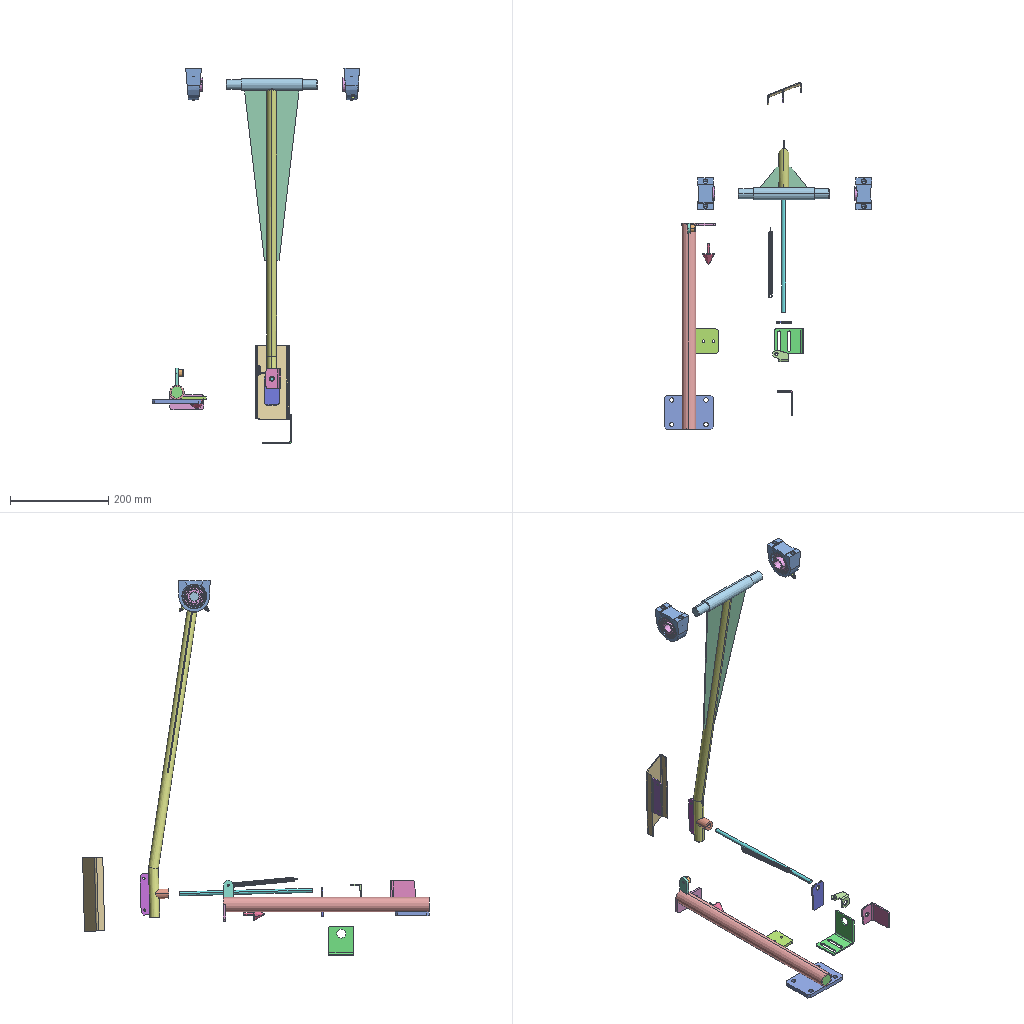Assembly | SolidWorks | 27 different items | 47 placed | box 423 x 707 x 766 mm
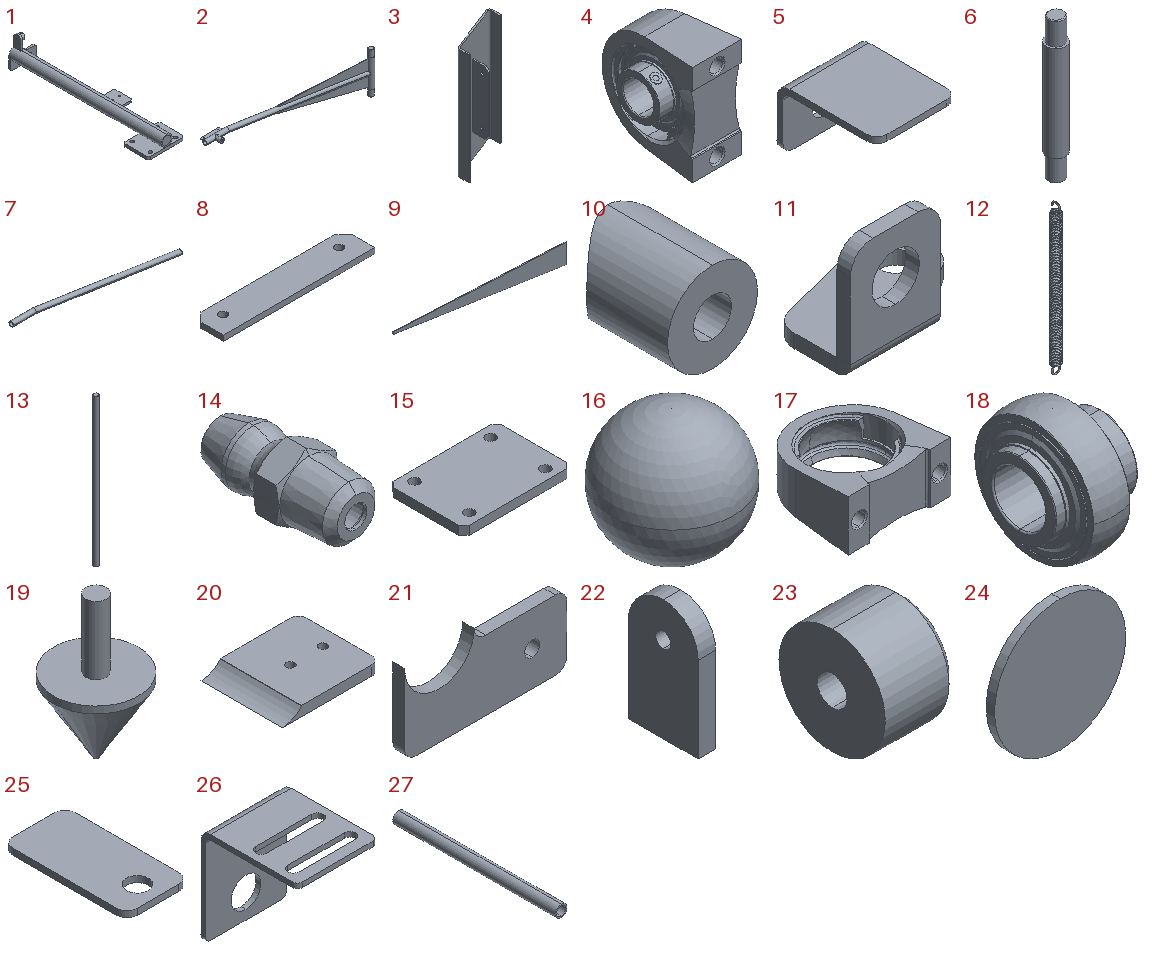Parts list (item | name | quantity | parent item | size | volume | features):
1 | (subassembly) | x1 | - | 110 x 420 x 84.5 mm | 197255 mm3 | -
2 | (subassembly) | x1 | - | 664 x 137.209 x 185 mm | 198892 mm3 | features RefAxis 1
3 | (subassembly) | x1 | - | 69 x 41.139 x 150 mm | 33678 mm3 | -
4 | (subassembly) | x2 | - | 34.3 x 65 x 65 mm | 66950 mm3 | features AEMSimFeature 1
5 | - | x1 | - | 40 x 50 x 30 mm | 8684 mm3 | features EdgeFlange 1, Fillet 1, FlatPattern 1, ICE 1, SMBaseFlange 1, SheetMetal 1
6 | - | x1 | - | 25 x 25 x 185 mm | 80148 mm3 | features ICE 2, Chamfer 1, Extrusion 1
7 | - | x1 | - | 645.85 x 115.746 x 20 mm | 73442 mm3 | features Cut 1, Sweep 1
8 | - | x1 | - | 85 x 17.5 x 3 mm | 4292 mm3 | features Cut 1, Extrusion 1
9 | - | x2 | in 2 | 345.03 x 62.746 x 45 mm | 17700 mm3 | features Extrusion 1
10 | - | x1 | - | 20 x 23.367 x 20 mm | 4988 mm3 | features 3DProfileFeature 1, Extrusion 1, HoleWzd 1
11 | - | x1 | - | 32.5 x 22.5 x 25 mm | 2512 mm3 | features EdgeFlange 1, Fillet 1, FlatPattern 1, ICE 1, SMBaseFlange 1, SheetMetal 1
12 | - | x1 | - | 8.5 x 8.5 x 143.5 mm | 2760 mm3 | features Sweep 5, 3DProfileFeature 4, Helix 1
13 | - | x1 | - | 8.5 x 8.5 x 271.5 mm | 15400 mm3 | features Chamfer 1, Extrusion 1
14 | - | x2 | in 4 | 7.001 x 16.4 x 8.083 mm | 360.824 mm3 | features BaseBody 1
15 | - | x1 | in 1 | 100 x 70 x 8 mm | 53564 mm3 | features Chamfer 1, Cut 1, Extrusion 1
16 | - | x16 | in 4 | 7.938 x 7.938 x 7.938 mm | 261.898 mm3 | features BaseBody 1
17 | - | x2 | in 4 | 65 x 65 x 32 mm | 47548 mm3 | features BaseBody 1
18 | - | x2 | in 4 | 31 x 47 x 47 mm | 16946 mm3 | features BaseBody 1
19 | - | x1 | - | 25 x 25 x 42 mm | 4956 mm3 | features Extrusion 1, ICE 1, Revolution 1
20 | - | x1 | in 1 | 60 x 50 x 6 mm | 15185 mm3 | features 3DProfileFeature 1, Extrusion 1, HoleWzd 1, ICE 1
21 | - | x1 | in 1 | 70 x 5 x 35 mm | 9263 mm3 | features Cut 1, Extrusion 1, Fillet 1, ICE 1
22 | - | x1 | in 1 | 5 x 20 x 34.5 mm | 3166 mm3 | features 3DProfileFeature 1, Extrusion 1, HoleWzd 1
23 | - | x1 | in 1 | 10 x 15 x 15 mm | 1606 mm3 | features 3DProfileFeature 1, Chamfer 1, Extrusion 1, HoleWzd 1
24 | - | x1 | in 1 | 23.6 x 1.5 x 23.6 mm | 656.153 mm3 | features Extrusion 1
25 | - | x1 | - | 30 x 60 x 3 mm | 5076 mm3 | features Extrusion 1
26 | - | x1 | - | 50 x 60 x 60 mm | 14730 mm3 | features ICE 2, EdgeFlange 1, Fillet 1, FlatPattern 1, SMBaseFlange 1, SheetMetal 1
27 | - | x1 | in 1 | 30 x 420 x 30 mm | 113158 mm3 | features Extrusion 1
Mates (type | each side: item.copy, entity, surface, feature):
In the top assembly
Concentric | 25.1 edge | 11.1 face cylinder Cut-Extrude1
Concentric | 11.1 face cylinder Cut-Extrude1 | 5.1 face cylinder Cut-Extrude1
Concentric | 11.1 face cylinder Cut-Extrude1 | 13.1 face cylinder Boss-Extrude1 | 2 times
Parallel | 25.1 face plane Boss-Extrude1 | 11.1 face plane Base-Flange1
Parallel | 11.1 face plane Edge-Flange1 | 5.1 face plane Edge-Flange1
Coincident | 21.1 face plane Boss-Extrude1 | 19.1 face plane Boss-Extrude2
Concentric | 21.1 face cylinder Cut-Extrude1 | 19.1 face cylinder Boss-Extrude1
Coincident | 20.1 face plane Boss-Extrude1 | 26.1 face plane Base-Flange1
Slot | 26.1 face cylinder Cut-Extrude1 | 20.1 face cylinder M6 Tapped Hole1 | 2 times
Coincident | 17.1 face plane SYF 504 -h(1) | 17.2 face plane SYF 504 -h(1)
Parallel | 15.1 face plane Boss-Extrude1 | 17.2 face plane SYF 504 -h(1)
In subassembly 2
Coincident | 9.1 face plane Boss-Extrude1 | 9.2 face plane Boss-Extrude1 | 2 times